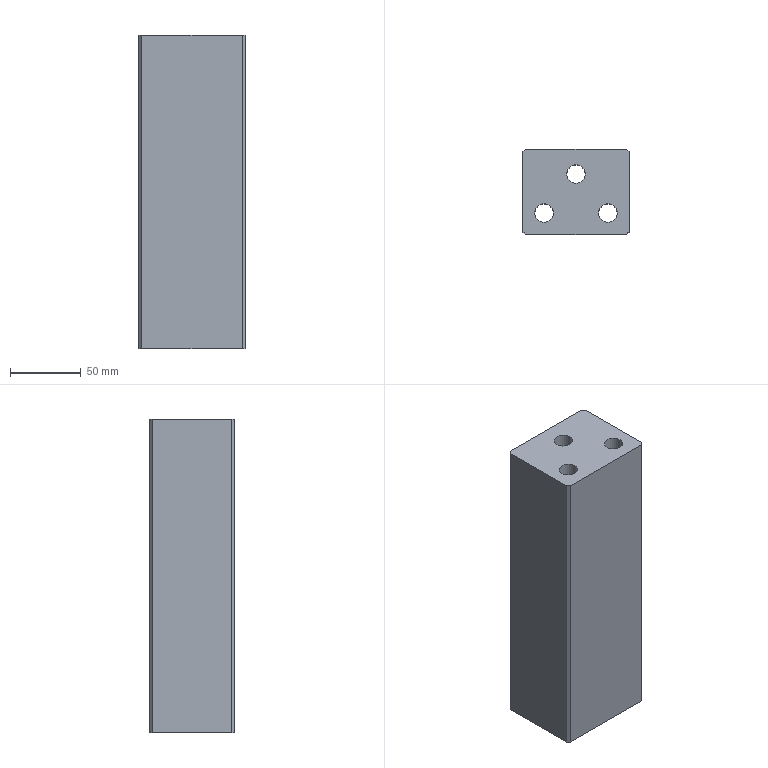Part | STEP file | lll_id1906_x_t | 1 solid | 25 faces | box 75 x 60 x 221 mm | volume 827204 mm3 | plane 13 | cylinder 9 | cone 3 | commonest cylinder face diameters 10.505 x3 13 x3 20 x3
STEP:
#1=CARTESIAN_POINT('',(3893.435,-384.5,46.5));
#2=VERTEX_POINT('',#1);
#3=CARTESIAN_POINT('',(3899.935,-384.5,46.5));
#4=DIRECTION('',(0.,0.,1.));
#5=DIRECTION('',(-1.,0.,0.));
#6=AXIS2_PLACEMENT_3D('',#3,#4,#5);
#7=CIRCLE('',#6,6.5);
#8=EDGE_CURVE('',#2,#2,#7,.T.);
#9=ORIENTED_EDGE('',*,*,#8,.T.);
#10=EDGE_LOOP('',(#9));
#11=FACE_BOUND('',#10,.T.);
#12=CARTESIAN_POINT('',(3889.935,-384.5,46.5));
#13=VERTEX_POINT('',#12);
#14=CARTESIAN_POINT('',(3899.935,-384.5,46.5));
#15=DIRECTION('',(0.,0.,1.));
#16=DIRECTION('',(-1.,0.,0.));
#17=AXIS2_PLACEMENT_3D('',#14,#15,#16);
#18=CIRCLE('',#17,10.);
#19=EDGE_CURVE('',#13,#13,#18,.T.);
#20=ORIENTED_EDGE('',*,*,#19,.F.);
#21=EDGE_LOOP('',(#20));
#22=FACE_BOUND('',#21,.T.);
#23=CARTESIAN_POINT('',(3899.935,-384.5,46.5));
#24=DIRECTION('',(0.,0.,1.));
#25=DIRECTION('',(1.,0.,0.));
#26=AXIS2_PLACEMENT_3D('',#23,#24,#25);
#27=PLANE('',#26);
#28=ADVANCED_FACE('',(#11,#22),#27,.F.);
#29=CARTESIAN_POINT('',(3870.935,-412.,46.5));
#30=VERTEX_POINT('',#29);
#31=CARTESIAN_POINT('',(3877.435,-412.,46.5));
#32=DIRECTION('',(0.,0.,1.));
#33=DIRECTION('',(-1.,0.,0.));
#34=AXIS2_PLACEMENT_3D('',#31,#32,#33);
#35=CIRCLE('',#34,6.5);
#36=EDGE_CURVE('',#30,#30,#35,.T.);
#37=ORIENTED_EDGE('',*,*,#36,.T.);
#38=EDGE_LOOP('',(#37));
#39=FACE_BOUND('',#38,.T.);
#40=CARTESIAN_POINT('',(3867.435,-412.,46.5));
#41=VERTEX_POINT('',#40);
#42=CARTESIAN_POINT('',(3877.435,-412.,46.5));
#43=DIRECTION('',(0.,0.,1.));
#44=DIRECTION('',(-1.,0.,0.));
#45=AXIS2_PLACEMENT_3D('',#42,#43,#44);
#46=CIRCLE('',#45,10.);
#47=EDGE_CURVE('',#41,#41,#46,.T.);
#48=ORIENTED_EDGE('',*,*,#47,.F.);
#49=EDGE_LOOP('',(#48));
#50=FACE_BOUND('',#49,.T.);
#51=CARTESIAN_POINT('',(3877.435,-412.,46.5));
#52=DIRECTION('',(0.,0.,1.));
#53=DIRECTION('',(1.,0.,0.));
#54=AXIS2_PLACEMENT_3D('',#51,#52,#53);
#55=PLANE('',#54);
#56=ADVANCED_FACE('',(#39,#50),#55,.F.);
#57=CARTESIAN_POINT('',(3937.435,-425.,-78.5));
#58=VERTEX_POINT('',#57);
#59=CARTESIAN_POINT('',(3937.435,-369.,-78.5));
#60=VERTEX_POINT('',#59);
#61=CARTESIAN_POINT('',(3937.435,-411.5,-78.5));
#62=DIRECTION('',(0.,1.,0.));
#63=VECTOR('',#62,1.);
#64=LINE('',#61,#63);
#65=EDGE_CURVE('',#58,#60,#64,.T.);
#66=ORIENTED_EDGE('',*,*,#65,.T.);
#67=CARTESIAN_POINT('',(3937.435,-369.,142.5));
#68=VERTEX_POINT('',#67);
#69=CARTESIAN_POINT('',(3937.435,-369.,129.));
#70=DIRECTION('',(0.,0.,1.));
#71=VECTOR('',#70,1.);
#72=LINE('',#69,#71);
#73=EDGE_CURVE('',#60,#68,#72,.T.);
#74=ORIENTED_EDGE('',*,*,#73,.T.);
#75=CARTESIAN_POINT('',(3937.435,-425.,142.5));
#76=VERTEX_POINT('',#75);
#77=CARTESIAN_POINT('',(3937.435,-411.5,142.5));
#78=DIRECTION('',(0.,1.,0.));
#79=VECTOR('',#78,1.);
#80=LINE('',#77,#79);
#81=EDGE_CURVE('',#76,#68,#80,.T.);
#82=ORIENTED_EDGE('',*,*,#81,.F.);
#83=CARTESIAN_POINT('',(3937.435,-425.,129.));
#84=DIRECTION('',(0.,0.,-1.));
#85=VECTOR('',#84,1.);
#86=LINE('',#83,#85);
#87=EDGE_CURVE('',#76,#58,#86,.T.);
#88=ORIENTED_EDGE('',*,*,#87,.T.);
#89=EDGE_LOOP('',(#66,#74,#82,#88));
#90=FACE_OUTER_BOUND('',#89,.T.);
#91=CARTESIAN_POINT('',(3937.435,-411.5,129.));
#92=DIRECTION('',(-1.,0.,0.));
#93=DIRECTION('',(0.,0.,1.));
#94=AXIS2_PLACEMENT_3D('',#91,#92,#93);
#95=PLANE('',#94);
#96=ADVANCED_FACE('',(#90),#95,.F.);
#97=CARTESIAN_POINT('',(3864.435,-427.,-78.5));
#98=VERTEX_POINT('',#97);
#99=CARTESIAN_POINT('',(3935.435,-427.,-78.5));
#100=VERTEX_POINT('',#99);
#101=CARTESIAN_POINT('',(3873.935,-427.,-78.5));
#102=DIRECTION('',(1.,0.,0.));
#103=VECTOR('',#102,1.);
#104=LINE('',#101,#103);
#105=EDGE_CURVE('',#98,#100,#104,.T.);
#106=ORIENTED_EDGE('',*,*,#105,.T.);
#107=CARTESIAN_POINT('',(3935.435,-427.,142.5));
#108=VERTEX_POINT('',#107);
#109=CARTESIAN_POINT('',(3935.435,-427.,129.));
#110=DIRECTION('',(0.,0.,1.));
#111=VECTOR('',#110,1.);
#112=LINE('',#109,#111);
#113=EDGE_CURVE('',#100,#108,#112,.T.);
#114=ORIENTED_EDGE('',*,*,#113,.T.);
#115=CARTESIAN_POINT('',(3864.435,-427.,142.5));
#116=VERTEX_POINT('',#115);
#117=CARTESIAN_POINT('',(3873.935,-427.,142.5));
#118=DIRECTION('',(1.,0.,0.));
#119=VECTOR('',#118,1.);
#120=LINE('',#117,#119);
#121=EDGE_CURVE('',#116,#108,#120,.T.);
#122=ORIENTED_EDGE('',*,*,#121,.F.);
#123=CARTESIAN_POINT('',(3864.435,-427.,129.));
#124=DIRECTION('',(0.,0.,-1.));
#125=VECTOR('',#124,1.);
#126=LINE('',#123,#125);
#127=EDGE_CURVE('',#116,#98,#126,.T.);
#128=ORIENTED_EDGE('',*,*,#127,.T.);
#129=EDGE_LOOP('',(#106,#114,#122,#128));
#130=FACE_OUTER_BOUND('',#129,.T.);
#131=CARTESIAN_POINT('',(3873.935,-427.,129.));
#132=DIRECTION('',(0.,1.,0.));
#133=DIRECTION('',(-1.,0.,0.));
#134=AXIS2_PLACEMENT_3D('',#131,#132,#133);
#135=PLANE('',#134);
#136=ADVANCED_FACE('',(#130),#135,.F.);
#137=CARTESIAN_POINT('',(3862.435,-369.,142.5));
#138=VERTEX_POINT('',#137);
#139=CARTESIAN_POINT('',(3862.435,-425.,142.5));
#140=VERTEX_POINT('',#139);
#141=CARTESIAN_POINT('',(3862.435,-372.5,142.5));
#142=DIRECTION('',(0.,-1.,0.));
#143=VECTOR('',#142,1.);
#144=LINE('',#141,#143);
#145=EDGE_CURVE('',#138,#140,#144,.T.);
#146=ORIENTED_EDGE('',*,*,#145,.F.);
#147=CARTESIAN_POINT('',(3862.435,-369.,-78.5));
#148=VERTEX_POINT('',#147);
#149=CARTESIAN_POINT('',(3862.435,-369.,129.));
#150=DIRECTION('',(0.,0.,-1.));
#151=VECTOR('',#150,1.);
#152=LINE('',#149,#151);
#153=EDGE_CURVE('',#138,#148,#152,.T.);
#154=ORIENTED_EDGE('',*,*,#153,.T.);
#155=CARTESIAN_POINT('',(3862.435,-425.,-78.5));
#156=VERTEX_POINT('',#155);
#157=CARTESIAN_POINT('',(3862.435,-372.5,-78.5));
#158=DIRECTION('',(0.,-1.,0.));
#159=VECTOR('',#158,1.);
#160=LINE('',#157,#159);
#161=EDGE_CURVE('',#148,#156,#160,.T.);
#162=ORIENTED_EDGE('',*,*,#161,.T.);
#163=CARTESIAN_POINT('',(3862.435,-425.,129.));
#164=DIRECTION('',(0.,0.,1.));
#165=VECTOR('',#164,1.);
#166=LINE('',#163,#165);
#167=EDGE_CURVE('',#156,#140,#166,.T.);
#168=ORIENTED_EDGE('',*,*,#167,.T.);
#169=EDGE_LOOP('',(#146,#154,#162,#168));
#170=FACE_OUTER_BOUND('',#169,.T.);
#171=CARTESIAN_POINT('',(3862.435,-372.5,129.));
#172=DIRECTION('',(1.,0.,0.));
#173=DIRECTION('',(0.,0.,-1.));
#174=AXIS2_PLACEMENT_3D('',#171,#172,#173);
#175=PLANE('',#174);
#176=ADVANCED_FACE('',(#170),#175,.F.);
#177=CARTESIAN_POINT('',(3935.435,-367.,142.5));
#178=VERTEX_POINT('',#177);
#179=CARTESIAN_POINT('',(3864.435,-367.,142.5));
#180=VERTEX_POINT('',#179);
#181=CARTESIAN_POINT('',(3925.935,-367.,142.5));
#182=DIRECTION('',(-1.,0.,0.));
#183=VECTOR('',#182,1.);
#184=LINE('',#181,#183);
#185=EDGE_CURVE('',#178,#180,#184,.T.);
#186=ORIENTED_EDGE('',*,*,#185,.F.);
#187=CARTESIAN_POINT('',(3935.435,-367.,-78.5));
#188=VERTEX_POINT('',#187);
#189=CARTESIAN_POINT('',(3935.435,-367.,129.));
#190=DIRECTION('',(0.,0.,-1.));
#191=VECTOR('',#190,1.);
#192=LINE('',#189,#191);
#193=EDGE_CURVE('',#178,#188,#192,.T.);
#194=ORIENTED_EDGE('',*,*,#193,.T.);
#195=CARTESIAN_POINT('',(3864.435,-367.,-78.5));
#196=VERTEX_POINT('',#195);
#197=CARTESIAN_POINT('',(3925.935,-367.,-78.5));
#198=DIRECTION('',(-1.,0.,0.));
#199=VECTOR('',#198,1.);
#200=LINE('',#197,#199);
#201=EDGE_CURVE('',#188,#196,#200,.T.);
#202=ORIENTED_EDGE('',*,*,#201,.T.);
#203=CARTESIAN_POINT('',(3864.435,-367.,129.));
#204=DIRECTION('',(0.,0.,1.));
#205=VECTOR('',#204,1.);
#206=LINE('',#203,#205);
#207=EDGE_CURVE('',#196,#180,#206,.T.);
#208=ORIENTED_EDGE('',*,*,#207,.T.);
#209=EDGE_LOOP('',(#186,#194,#202,#208));
#210=FACE_OUTER_BOUND('',#209,.T.);
#211=CARTESIAN_POINT('',(3925.935,-367.,129.));
#212=DIRECTION('',(0.,-1.,0.));
#213=DIRECTION('',(0.,0.,-1.));
#214=AXIS2_PLACEMENT_3D('',#211,#212,#213);
#215=PLANE('',#214);
#216=ADVANCED_FACE('',(#210),#215,.F.);
#217=CARTESIAN_POINT('',(3906.435,-384.5,142.5));
#218=VERTEX_POINT('',#217);
#219=CARTESIAN_POINT('',(3899.935,-384.5,142.5));
#220=DIRECTION('',(0.,0.,-1.));
#221=DIRECTION('',(1.,0.,0.));
#222=AXIS2_PLACEMENT_3D('',#219,#220,#221);
#223=CIRCLE('',#222,6.5);
#224=EDGE_CURVE('',#218,#218,#223,.T.);
#225=ORIENTED_EDGE('',*,*,#224,.F.);
#226=EDGE_LOOP('',(#225));
#227=FACE_BOUND('',#226,.T.);
#228=ORIENTED_EDGE('',*,*,#8,.F.);
#229=EDGE_LOOP('',(#228));
#230=FACE_BOUND('',#229,.T.);
#231=CARTESIAN_POINT('',(3899.935,-384.5,186.5));
#232=DIRECTION('',(0.,0.,1.));
#233=DIRECTION('',(1.,0.,0.));
#234=AXIS2_PLACEMENT_3D('',#231,#232,#233);
#235=CYLINDRICAL_SURFACE('',#234,6.5);
#236=ADVANCED_FACE('',(#227,#230),#235,.F.);
#237=CARTESIAN_POINT('',(3883.935,-412.,142.5));
#238=VERTEX_POINT('',#237);
#239=CARTESIAN_POINT('',(3877.435,-412.,142.5));
#240=DIRECTION('',(0.,0.,-1.));
#241=DIRECTION('',(1.,0.,0.));
#242=AXIS2_PLACEMENT_3D('',#239,#240,#241);
#243=CIRCLE('',#242,6.5);
#244=EDGE_CURVE('',#238,#238,#243,.T.);
#245=ORIENTED_EDGE('',*,*,#244,.F.);
#246=EDGE_LOOP('',(#245));
#247=FACE_BOUND('',#246,.T.);
#248=ORIENTED_EDGE('',*,*,#36,.F.);
#249=EDGE_LOOP('',(#248));
#250=FACE_BOUND('',#249,.T.);
#251=CARTESIAN_POINT('',(3877.435,-412.,186.5));
#252=DIRECTION('',(0.,0.,1.));
#253=DIRECTION('',(1.,0.,0.));
#254=AXIS2_PLACEMENT_3D('',#251,#252,#253);
#255=CYLINDRICAL_SURFACE('',#254,6.5);
#256=ADVANCED_FACE('',(#247,#250),#255,.F.);
#257=CARTESIAN_POINT('',(3928.935,-412.,142.5));
#258=VERTEX_POINT('',#257);
#259=CARTESIAN_POINT('',(3922.435,-412.,142.5));
#260=DIRECTION('',(0.,0.,1.));
#261=DIRECTION('',(1.,0.,0.));
#262=AXIS2_PLACEMENT_3D('',#259,#260,#261);
#263=CIRCLE('',#262,6.5);
#264=EDGE_CURVE('',#258,#258,#263,.T.);
#265=ORIENTED_EDGE('',*,*,#264,.F.);
#266=EDGE_LOOP('',(#265));
#267=FACE_BOUND('',#266,.T.);
#268=ORIENTED_EDGE('',*,*,#244,.T.);
#269=EDGE_LOOP('',(#268));
#270=FACE_BOUND('',#269,.T.);
#271=ORIENTED_EDGE('',*,*,#224,.T.);
#272=EDGE_LOOP('',(#271));
#273=FACE_BOUND('',#272,.T.);
#274=ORIENTED_EDGE('',*,*,#81,.T.);
#275=CARTESIAN_POINT('',(3915.545,-347.11,142.5));
#276=DIRECTION('',(-0.7071,0.7071,0.));
#277=VECTOR('',#276,1.);
#278=LINE('',#275,#277);
#279=EDGE_CURVE('',#68,#178,#278,.T.);
#280=ORIENTED_EDGE('',*,*,#279,.T.);
#281=ORIENTED_EDGE('',*,*,#185,.T.);
#282=CARTESIAN_POINT('',(4034.342,-197.094,142.5));
#283=DIRECTION('',(-0.7071,-0.7071,0.));
#284=VECTOR('',#283,1.);
#285=LINE('',#282,#284);
#286=EDGE_CURVE('',#180,#138,#285,.T.);
#287=ORIENTED_EDGE('',*,*,#286,.T.);
#288=ORIENTED_EDGE('',*,*,#145,.T.);
#289=CARTESIAN_POINT('',(3850.045,-412.61,142.5));
#290=DIRECTION('',(0.7071,-0.7071,0.));
#291=VECTOR('',#290,1.);
#292=LINE('',#289,#291);
#293=EDGE_CURVE('',#140,#116,#292,.T.);
#294=ORIENTED_EDGE('',*,*,#293,.T.);
#295=ORIENTED_EDGE('',*,*,#121,.T.);
#296=CARTESIAN_POINT('',(4099.842,-262.594,142.5));
#297=DIRECTION('',(0.7071,0.7071,0.));
#298=VECTOR('',#297,1.);
#299=LINE('',#296,#298);
#300=EDGE_CURVE('',#108,#76,#299,.T.);
#301=ORIENTED_EDGE('',*,*,#300,.T.);
#302=EDGE_LOOP('',(#274,#280,#281,#287,#288,#294,#295,#301));
#303=FACE_BOUND('',#302,.T.);
#304=CARTESIAN_POINT('',(4049.951,-212.704,142.5));
#305=DIRECTION('',(0.,0.,1.));
#306=DIRECTION('',(1.,0.,0.));
#307=AXIS2_PLACEMENT_3D('',#304,#305,#306);
#308=PLANE('',#307);
#309=ADVANCED_FACE('',(#267,#270,#273,#303),#308,.T.);
#310=ORIENTED_EDGE('',*,*,#19,.T.);
#311=EDGE_LOOP('',(#310));
#312=FACE_BOUND('',#311,.T.);
#313=CARTESIAN_POINT('',(3909.935,-384.5,-78.5));
#314=VERTEX_POINT('',#313);
#315=CARTESIAN_POINT('',(3899.935,-384.5,-78.5));
#316=DIRECTION('',(0.,0.,-1.));
#317=DIRECTION('',(1.,0.,0.));
#318=AXIS2_PLACEMENT_3D('',#315,#316,#317);
#319=CIRCLE('',#318,10.);
#320=EDGE_CURVE('',#314,#314,#319,.T.);
#321=ORIENTED_EDGE('',*,*,#320,.T.);
#322=EDGE_LOOP('',(#321));
#323=FACE_BOUND('',#322,.T.);
#324=CARTESIAN_POINT('',(3899.935,-384.5,-83.5));
#325=DIRECTION('',(0.,0.,1.));
#326=DIRECTION('',(1.,0.,0.));
#327=AXIS2_PLACEMENT_3D('',#324,#325,#326);
#328=CYLINDRICAL_SURFACE('',#327,10.);
#329=ADVANCED_FACE('',(#312,#323),#328,.F.);
#330=ORIENTED_EDGE('',*,*,#47,.T.);
#331=EDGE_LOOP('',(#330));
#332=FACE_BOUND('',#331,.T.);
#333=CARTESIAN_POINT('',(3887.435,-412.,-78.5));
#334=VERTEX_POINT('',#333);
#335=CARTESIAN_POINT('',(3877.435,-412.,-78.5));
#336=DIRECTION('',(0.,0.,-1.));
#337=DIRECTION('',(1.,0.,0.));
#338=AXIS2_PLACEMENT_3D('',#335,#336,#337);
#339=CIRCLE('',#338,10.);
#340=EDGE_CURVE('',#334,#334,#339,.T.);
#341=ORIENTED_EDGE('',*,*,#340,.T.);
#342=EDGE_LOOP('',(#341));
#343=FACE_BOUND('',#342,.T.);
#344=CARTESIAN_POINT('',(3877.435,-412.,-83.5));
#345=DIRECTION('',(0.,0.,1.));
#346=DIRECTION('',(1.,0.,0.));
#347=AXIS2_PLACEMENT_3D('',#344,#345,#346);
#348=CYLINDRICAL_SURFACE('',#347,10.);
#349=ADVANCED_FACE('',(#332,#343),#348,.F.);
#350=CARTESIAN_POINT('',(3916.683,-381.5,-78.5));
#351=VERTEX_POINT('',#350);
#352=CARTESIAN_POINT('',(3921.935,-381.5,-78.5));
#353=DIRECTION('',(0.,0.,1.));
#354=DIRECTION('',(-1.,0.,0.));
#355=AXIS2_PLACEMENT_3D('',#352,#353,#354);
#356=CIRCLE('',#355,5.253);
#357=EDGE_CURVE('',#351,#351,#356,.T.);
#358=ORIENTED_EDGE('',*,*,#357,.T.);
#359=EDGE_LOOP('',(#358));
#360=FACE_BOUND('',#359,.T.);
#361=CARTESIAN_POINT('',(3872.683,-381.5,-78.5));
#362=VERTEX_POINT('',#361);
#363=CARTESIAN_POINT('',(3877.935,-381.5,-78.5));
#364=DIRECTION('',(0.,0.,1.));
#365=DIRECTION('',(-1.,0.,0.));
#366=AXIS2_PLACEMENT_3D('',#363,#364,#365);
#367=CIRCLE('',#366,5.253);
#368=EDGE_CURVE('',#362,#362,#367,.T.);
#369=ORIENTED_EDGE('',*,*,#368,.T.);
#370=EDGE_LOOP('',(#369));
#371=FACE_BOUND('',#370,.T.);
#372=CARTESIAN_POINT('',(3894.683,-407.5,-78.5));
#373=VERTEX_POINT('',#372);
#374=CARTESIAN_POINT('',(3899.935,-407.5,-78.5));
#375=DIRECTION('',(0.,0.,1.));
#376=DIRECTION('',(-1.,0.,0.));
#377=AXIS2_PLACEMENT_3D('',#374,#375,#376);
#378=CIRCLE('',#377,5.253);
#379=EDGE_CURVE('',#373,#373,#378,.T.);
#380=ORIENTED_EDGE('',*,*,#379,.T.);
#381=EDGE_LOOP('',(#380));
#382=FACE_BOUND('',#381,.T.);
#383=CARTESIAN_POINT('',(3932.435,-412.,-78.5));
#384=VERTEX_POINT('',#383);
#385=CARTESIAN_POINT('',(3922.435,-412.,-78.5));
#386=DIRECTION('',(0.,0.,1.));
#387=DIRECTION('',(1.,0.,0.));
#388=AXIS2_PLACEMENT_3D('',#385,#386,#387);
#389=CIRCLE('',#388,10.);
#390=EDGE_CURVE('',#384,#384,#389,.T.);
#391=ORIENTED_EDGE('',*,*,#390,.T.);
#392=EDGE_LOOP('',(#391));
#393=FACE_BOUND('',#392,.T.);
#394=ORIENTED_EDGE('',*,*,#340,.F.);
#395=EDGE_LOOP('',(#394));
#396=FACE_BOUND('',#395,.T.);
#397=ORIENTED_EDGE('',*,*,#320,.F.);
#398=EDGE_LOOP('',(#397));
#399=FACE_BOUND('',#398,.T.);
#400=ORIENTED_EDGE('',*,*,#201,.F.);
#401=CARTESIAN_POINT('',(3937.435,-369.,-78.5));
#402=DIRECTION('',(0.7071,-0.7071,0.));
#403=VECTOR('',#402,1.);
#404=LINE('',#401,#403);
#405=EDGE_CURVE('',#188,#60,#404,.T.);
#406=ORIENTED_EDGE('',*,*,#405,.T.);
#407=ORIENTED_EDGE('',*,*,#65,.F.);
#408=CARTESIAN_POINT('',(3935.435,-427.,-78.5));
#409=DIRECTION('',(-0.7071,-0.7071,0.));
#410=VECTOR('',#409,1.);
#411=LINE('',#408,#410);
#412=EDGE_CURVE('',#58,#100,#411,.T.);
#413=ORIENTED_EDGE('',*,*,#412,.T.);
#414=ORIENTED_EDGE('',*,*,#105,.F.);
#415=CARTESIAN_POINT('',(3862.435,-425.,-78.5));
#416=DIRECTION('',(-0.7071,0.7071,0.));
#417=VECTOR('',#416,1.);
#418=LINE('',#415,#417);
#419=EDGE_CURVE('',#98,#156,#418,.T.);
#420=ORIENTED_EDGE('',*,*,#419,.T.);
#421=ORIENTED_EDGE('',*,*,#161,.F.);
#422=CARTESIAN_POINT('',(3864.435,-367.,-78.5));
#423=DIRECTION('',(0.7071,0.7071,0.));
#424=VECTOR('',#423,1.);
#425=LINE('',#422,#424);
#426=EDGE_CURVE('',#148,#196,#425,.T.);
#427=ORIENTED_EDGE('',*,*,#426,.T.);
#428=EDGE_LOOP('',(#400,#406,#407,#413,#414,#420,#421,#427));
#429=FACE_BOUND('',#428,.T.);
#430=CARTESIAN_POINT('',(3870.935,-369.5,-78.5));
#431=DIRECTION('',(0.,0.,1.));
#432=DIRECTION('',(1.,0.,0.));
#433=AXIS2_PLACEMENT_3D('',#430,#431,#432);
#434=PLANE('',#433);
#435=ADVANCED_FACE('',(#360,#371,#382,#393,#396,#399,#429),#434,.F.);
#436=CARTESIAN_POINT('',(3915.935,-412.,46.5));
#437=VERTEX_POINT('',#436);
#438=CARTESIAN_POINT('',(3922.435,-412.,46.5));
#439=DIRECTION('',(0.,0.,1.));
#440=DIRECTION('',(-1.,0.,0.));
#441=AXIS2_PLACEMENT_3D('',#438,#439,#440);
#442=CIRCLE('',#441,6.5);
#443=EDGE_CURVE('',#437,#437,#442,.T.);
#444=ORIENTED_EDGE('',*,*,#443,.T.);
#445=EDGE_LOOP('',(#444));
#446=FACE_BOUND('',#445,.T.);
#447=CARTESIAN_POINT('',(3912.435,-412.,46.5));
#448=VERTEX_POINT('',#447);
#449=CARTESIAN_POINT('',(3922.435,-412.,46.5));
#450=DIRECTION('',(0.,0.,1.));
#451=DIRECTION('',(-1.,0.,0.));
#452=AXIS2_PLACEMENT_3D('',#449,#450,#451);
#453=CIRCLE('',#452,10.);
#454=EDGE_CURVE('',#448,#448,#453,.T.);
#455=ORIENTED_EDGE('',*,*,#454,.F.);
#456=EDGE_LOOP('',(#455));
#457=FACE_BOUND('',#456,.T.);
#458=CARTESIAN_POINT('',(3922.435,-412.,46.5));
#459=DIRECTION('',(0.,0.,1.));
#460=DIRECTION('',(-1.,0.,0.));
#461=AXIS2_PLACEMENT_3D('',#458,#459,#460);
#462=PLANE('',#461);
#463=ADVANCED_FACE('',(#446,#457),#462,.F.);
#464=ORIENTED_EDGE('',*,*,#264,.T.);
#465=EDGE_LOOP('',(#464));
#466=FACE_BOUND('',#465,.T.);
#467=ORIENTED_EDGE('',*,*,#443,.F.);
#468=EDGE_LOOP('',(#467));
#469=FACE_BOUND('',#468,.T.);
#470=CARTESIAN_POINT('',(3922.435,-412.,186.5));
#471=DIRECTION('',(0.,0.,1.));
#472=DIRECTION('',(-1.,0.,0.));
#473=AXIS2_PLACEMENT_3D('',#470,#471,#472);
#474=CYLINDRICAL_SURFACE('',#473,6.5);
#475=ADVANCED_FACE('',(#466,#469),#474,.F.);
#476=ORIENTED_EDGE('',*,*,#454,.T.);
#477=EDGE_LOOP('',(#476));
#478=FACE_BOUND('',#477,.T.);
#479=ORIENTED_EDGE('',*,*,#390,.F.);
#480=EDGE_LOOP('',(#479));
#481=FACE_BOUND('',#480,.T.);
#482=CARTESIAN_POINT('',(3922.435,-412.,-83.5));
#483=DIRECTION('',(0.,0.,1.));
#484=DIRECTION('',(-1.,0.,0.));
#485=AXIS2_PLACEMENT_3D('',#482,#483,#484);
#486=CYLINDRICAL_SURFACE('',#485,10.);
#487=ADVANCED_FACE('',(#478,#481),#486,.F.);
#488=ORIENTED_EDGE('',*,*,#405,.F.);
#489=ORIENTED_EDGE('',*,*,#193,.F.);
#490=ORIENTED_EDGE('',*,*,#279,.F.);
#491=ORIENTED_EDGE('',*,*,#73,.F.);
#492=EDGE_LOOP('',(#488,#489,#490,#491));
#493=FACE_OUTER_BOUND('',#492,.T.);
#494=CARTESIAN_POINT('',(3937.435,-369.,129.));
#495=DIRECTION('',(-0.7071,-0.7071,0.));
#496=DIRECTION('',(0.,0.,1.));
#497=AXIS2_PLACEMENT_3D('',#494,#495,#496);
#498=PLANE('',#497);
#499=ADVANCED_FACE('',(#493),#498,.F.);
#500=ORIENTED_EDGE('',*,*,#412,.F.);
#501=ORIENTED_EDGE('',*,*,#87,.F.);
#502=ORIENTED_EDGE('',*,*,#300,.F.);
#503=ORIENTED_EDGE('',*,*,#113,.F.);
#504=EDGE_LOOP('',(#500,#501,#502,#503));
#505=FACE_OUTER_BOUND('',#504,.T.);
#506=CARTESIAN_POINT('',(3935.435,-427.,129.));
#507=DIRECTION('',(-0.7071,0.7071,0.));
#508=DIRECTION('',(0.,0.,1.));
#509=AXIS2_PLACEMENT_3D('',#506,#507,#508);
#510=PLANE('',#509);
#511=ADVANCED_FACE('',(#505),#510,.F.);
#512=ORIENTED_EDGE('',*,*,#426,.F.);
#513=ORIENTED_EDGE('',*,*,#153,.F.);
#514=ORIENTED_EDGE('',*,*,#286,.F.);
#515=ORIENTED_EDGE('',*,*,#207,.F.);
#516=EDGE_LOOP('',(#512,#513,#514,#515));
#517=FACE_OUTER_BOUND('',#516,.T.);
#518=CARTESIAN_POINT('',(3864.435,-367.,129.));
#519=DIRECTION('',(0.7071,-0.7071,0.));
#520=DIRECTION('',(0.,0.,1.));
#521=AXIS2_PLACEMENT_3D('',#518,#519,#520);
#522=PLANE('',#521);
#523=ADVANCED_FACE('',(#517),#522,.F.);
#524=ORIENTED_EDGE('',*,*,#419,.F.);
#525=ORIENTED_EDGE('',*,*,#127,.F.);
#526=ORIENTED_EDGE('',*,*,#293,.F.);
#527=ORIENTED_EDGE('',*,*,#167,.F.);
#528=EDGE_LOOP('',(#524,#525,#526,#527));
#529=FACE_OUTER_BOUND('',#528,.T.);
#530=CARTESIAN_POINT('',(3862.435,-425.,129.));
#531=DIRECTION('',(0.7071,0.7071,0.));
#532=DIRECTION('',(0.,0.,1.));
#533=AXIS2_PLACEMENT_3D('',#530,#531,#532);
#534=PLANE('',#533);
#535=ADVANCED_FACE('',(#529),#534,.F.);
#536=CARTESIAN_POINT('',(3894.683,-407.5,-43.746));
#537=VERTEX_POINT('',#536);
#538=CARTESIAN_POINT('',(3899.935,-407.5,-43.746));
#539=DIRECTION('',(0.,0.,1.));
#540=DIRECTION('',(-1.,0.,0.));
#541=AXIS2_PLACEMENT_3D('',#538,#539,#540);
#542=CIRCLE('',#541,5.253);
#543=EDGE_CURVE('',#537,#537,#542,.T.);
#544=ORIENTED_EDGE('',*,*,#543,.T.);
#545=EDGE_LOOP('',(#544));
#546=FACE_BOUND('',#545,.T.);
#547=ORIENTED_EDGE('',*,*,#379,.F.);
#548=EDGE_LOOP('',(#547));
#549=FACE_BOUND('',#548,.T.);
#550=CARTESIAN_POINT('',(3899.935,-407.5,-78.5));
#551=DIRECTION('',(0.,0.,1.));
#552=DIRECTION('',(-1.,0.,0.));
#553=AXIS2_PLACEMENT_3D('',#550,#551,#552);
#554=CYLINDRICAL_SURFACE('',#553,5.253);
#555=ADVANCED_FACE('',(#546,#549),#554,.F.);
#556=CARTESIAN_POINT('',(3899.935,-407.5,-38.494));
#557=VERTEX_POINT('',#556);
#558=VERTEX_LOOP('',#557);
#559=FACE_BOUND('',#558,.T.);
#560=ORIENTED_EDGE('',*,*,#543,.F.);
#561=EDGE_LOOP('',(#560));
#562=FACE_BOUND('',#561,.T.);
#563=CARTESIAN_POINT('',(3899.935,-407.5,-43.746));
#564=DIRECTION('',(0.,0.,-1.));
#565=DIRECTION('',(1.,0.,0.));
#566=AXIS2_PLACEMENT_3D('',#563,#564,#565);
#567=CONICAL_SURFACE('',#566,5.253,45.);
#568=ADVANCED_FACE('',(#559,#562),#567,.F.);
#569=CARTESIAN_POINT('',(3872.683,-381.5,-43.746));
#570=VERTEX_POINT('',#569);
#571=CARTESIAN_POINT('',(3877.935,-381.5,-43.746));
#572=DIRECTION('',(0.,0.,1.));
#573=DIRECTION('',(-1.,0.,0.));
#574=AXIS2_PLACEMENT_3D('',#571,#572,#573);
#575=CIRCLE('',#574,5.253);
#576=EDGE_CURVE('',#570,#570,#575,.T.);
#577=ORIENTED_EDGE('',*,*,#576,.T.);
#578=EDGE_LOOP('',(#577));
#579=FACE_BOUND('',#578,.T.);
#580=ORIENTED_EDGE('',*,*,#368,.F.);
#581=EDGE_LOOP('',(#580));
#582=FACE_BOUND('',#581,.T.);
#583=CARTESIAN_POINT('',(3877.935,-381.5,-78.5));
#584=DIRECTION('',(0.,0.,1.));
#585=DIRECTION('',(-1.,0.,0.));
#586=AXIS2_PLACEMENT_3D('',#583,#584,#585);
#587=CYLINDRICAL_SURFACE('',#586,5.253);
#588=ADVANCED_FACE('',(#579,#582),#587,.F.);
#589=CARTESIAN_POINT('',(3877.935,-381.5,-38.494));
#590=VERTEX_POINT('',#589);
#591=VERTEX_LOOP('',#590);
#592=FACE_BOUND('',#591,.T.);
#593=ORIENTED_EDGE('',*,*,#576,.F.);
#594=EDGE_LOOP('',(#593));
#595=FACE_BOUND('',#594,.T.);
#596=CARTESIAN_POINT('',(3877.935,-381.5,-43.746));
#597=DIRECTION('',(0.,0.,-1.));
#598=DIRECTION('',(1.,0.,0.));
#599=AXIS2_PLACEMENT_3D('',#596,#597,#598);
#600=CONICAL_SURFACE('',#599,5.253,45.);
#601=ADVANCED_FACE('',(#592,#595),#600,.F.);
#602=CARTESIAN_POINT('',(3916.683,-381.5,-43.746));
#603=VERTEX_POINT('',#602);
#604=CARTESIAN_POINT('',(3921.935,-381.5,-43.746));
#605=DIRECTION('',(0.,0.,1.));
#606=DIRECTION('',(-1.,0.,0.));
#607=AXIS2_PLACEMENT_3D('',#604,#605,#606);
#608=CIRCLE('',#607,5.253);
#609=EDGE_CURVE('',#603,#603,#608,.T.);
#610=ORIENTED_EDGE('',*,*,#609,.T.);
#611=EDGE_LOOP('',(#610));
#612=FACE_BOUND('',#611,.T.);
#613=ORIENTED_EDGE('',*,*,#357,.F.);
#614=EDGE_LOOP('',(#613));
#615=FACE_BOUND('',#614,.T.);
#616=CARTESIAN_POINT('',(3921.935,-381.5,-78.5));
#617=DIRECTION('',(0.,0.,1.));
#618=DIRECTION('',(-1.,0.,0.));
#619=AXIS2_PLACEMENT_3D('',#616,#617,#618);
#620=CYLINDRICAL_SURFACE('',#619,5.253);
#621=ADVANCED_FACE('',(#612,#615),#620,.F.);
#622=CARTESIAN_POINT('',(3921.935,-381.5,-38.494));
#623=VERTEX_POINT('',#622);
#624=VERTEX_LOOP('',#623);
#625=FACE_BOUND('',#624,.T.);
#626=ORIENTED_EDGE('',*,*,#609,.F.);
#627=EDGE_LOOP('',(#626));
#628=FACE_BOUND('',#627,.T.);
#629=CARTESIAN_POINT('',(3921.935,-381.5,-43.746));
#630=DIRECTION('',(0.,0.,-1.));
#631=DIRECTION('',(1.,0.,0.));
#632=AXIS2_PLACEMENT_3D('',#629,#630,#631);
#633=CONICAL_SURFACE('',#632,5.253,45.);
#634=ADVANCED_FACE('',(#625,#628),#633,.F.);
#635=CLOSED_SHELL('',(#28,#56,#96,#136,#176,#216,#236,#256,#309,#329,#349,#435,#463,#475,#487,#499,#511,#523,#535,#555,#568,#588,#601,#621,#634));
#636=MANIFOLD_SOLID_BREP('',#635);
#637=(LENGTH_UNIT()NAMED_UNIT(*)SI_UNIT(.MILLI.,.METRE.));
#638=UNCERTAINTY_MEASURE_WITH_UNIT(LENGTH_MEASURE(0.00002),#637,'','');
#639=(NAMED_UNIT(*)PLANE_ANGLE_UNIT()SI_UNIT($,.RADIAN.));
#640=PLANE_ANGLE_MEASURE_WITH_UNIT(PLANE_ANGLE_MEASURE(0.01745),#639);
#641=DIMENSIONAL_EXPONENTS(0.,0.,0.,0.,0.,0.,0.);
#642=(CONVERSION_BASED_UNIT('DEGREE',#640)NAMED_UNIT(#641)PLANE_ANGLE_UNIT());
#643=(NAMED_UNIT(*)SI_UNIT($,.STERADIAN.)SOLID_ANGLE_UNIT());
#644=(GEOMETRIC_REPRESENTATION_CONTEXT(3)GLOBAL_UNCERTAINTY_ASSIGNED_CONTEXT((#638))GLOBAL_UNIT_ASSIGNED_CONTEXT((#637,#642,#643))REPRESENTATION_CONTEXT('',''));
#645=ADVANCED_BREP_SHAPE_REPRESENTATION('',(#636),#644);